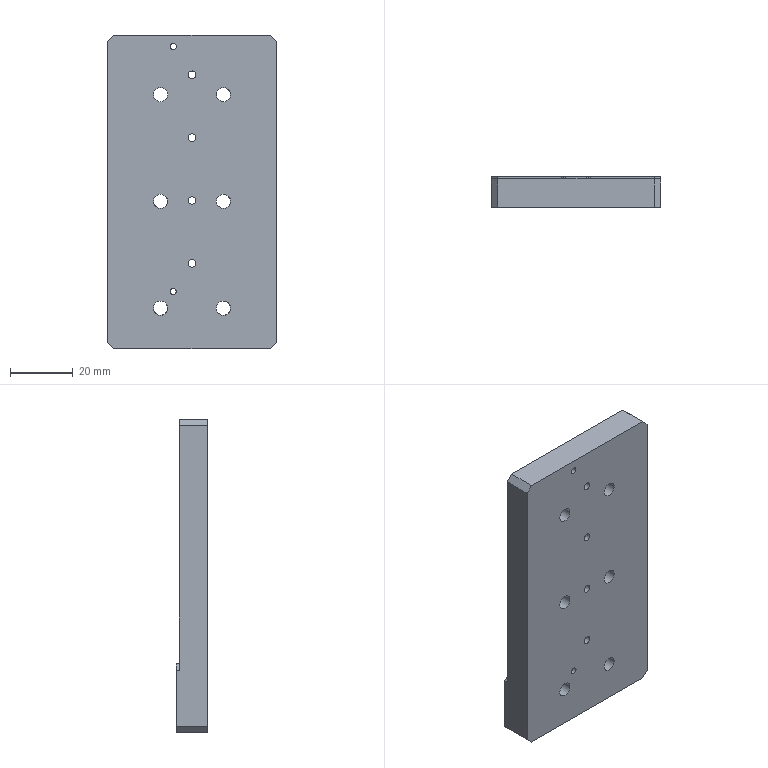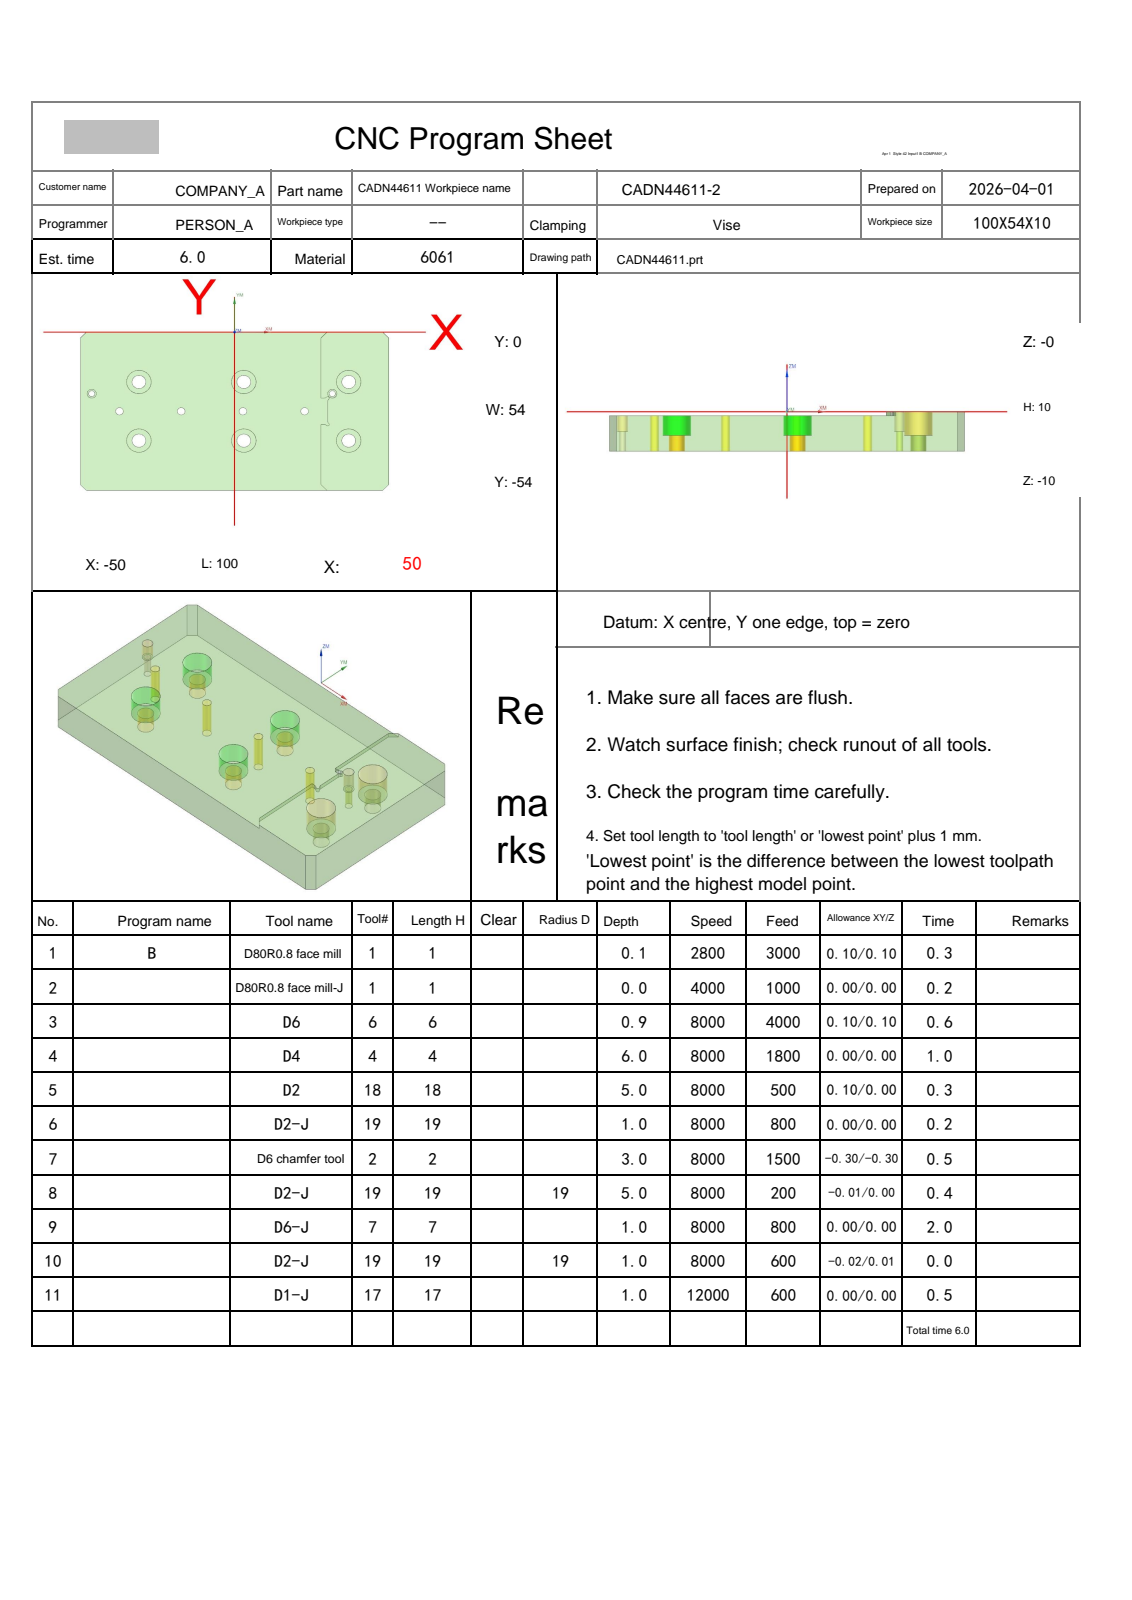NC program | NX | posted by the shop | part box 54 x 10 x 100 mm
Lines 1 to 1970 of 3760, first 1655 of 1968 lines:
%
O0001
(Machine time: 8.37 MIN)
(===Total Tool:8===)
(T1=D80R0.8 face mill D=80.  R=0.8  D-  H01 Z=-0.   )
(T6=D6      D=6.   R=0.   D-  H06 Z=-0.9  )
(T4=D4      D=4.   R=0.   D-  H04 Z=-6.   )
(T18=D2     D=2.   R=0.   D-  H18 Z=-5.   )
(T19=D2-J   D=2.   R=0.   D-  H19 Z=-5.   )
(T2=D6 chamfer tool   D=6.   R=0.   D-  H02 Z=-3.   )
(T7=D6-J    D=6.   R=0.   D7  H07 Z=-1.   )
(T17=D1-J   D=0.96 R=0.   D-  H17 Z=-1.   )
G80 G90 G17 G49 G40
G91 G28 Z0
M01
N1 T01 M06
(D80R0.8 face mill  D=80. R=0.8 H=01 ce=0.10 di=0.10)
G00 G90 G54 X-102.097 Y-27. M03 S2800
G43 H01 Z20.
M08
Z3.525
G01 Z1.525 F3000.
X-90.097
X90.097
X102.097
Z3.525
G00 X-102.097
Z3.05
G01 Z1.05
X-90.097
X90.097
X102.097
Z3.05
G00 X-102.097
Z2.575
G01 Z.575
X-90.097
X90.097
X102.097
Z2.575
G00 X-102.097
Z2.1
G01 Z.1
X-90.097
X90.097
X102.097
Z2.1
G00 Z20.
G91 G28 Z0.0
M05
M09
G91 G28 Z0.0
M01
N2 T01 M06
(D80R0.8 face mill-J  D=80. R=0.8 H=01 ce=0.00 di=0.00)
G00 G90 G54 X-101.999 Y-27. M03 S4000
G43 H01 Z20.
M08
Z2.
G01 Z0.0 F1000.
X-89.999
X89.999
X101.999
Z2.
G00 Z20.
G91 G28 Z0.0
M05
M09
G91 G28 Z0.0
M01
N3 T06 M06
(D6  D=6. R=0. H=06 ce=0.10 di=0.10)
G00 G90 G54 X-51.515 Y4.97 M03 S8000
G43 H06 Z11.801
M08
Z1.05
G01 Z-.45 F4000.
X-51.589 Y.569
G03 X-51.6 Y-.716 I76.489 J-1.285
G01 Y-25.601
G03 X-51.587 Y-27.001 I76.5 J0.0
X-51.6 Y-28.401 I76.487 J-1.4
G01 Y-53.291
G03 X-51.593 Y-54.325 I76.5 J.007
X-51.417 Y-54.74 I.6 J.008
G01 X-49.393 Y-56.764
G03 X-48.969 Y-56.94 I.424 J.424
G01 X-47.573
G03 X-47.033 Y-56.4 I0.0 J.54
G01 X-47.034 Y-56.377
G02 X-47.1 Y-53.291 I71.934 J3.093
G01 Y-28.401
G02 X-47.086 Y-27.001 I72. J0.0
X-47.1 Y-25.601 I71.986 J1.4
G01 Y-.716
G02 X-47.034 Y2.366 I72. J0.0
X-46.435 Y2.94 I.599 J-.026
G01 X-43.068
G02 X-42.529 Y2.4 I0.0 J-.54
G01 Y2.376
G03 X-42.6 Y-.716 I67.429 J-3.092
G01 Y-25.601
G03 X-42.585 Y-27.001 I67.5 J0.0
X-42.6 Y-28.401 I67.485 J-1.4
G01 Y-53.29
G03 X-42.53 Y-56.368 I67.5 J.006
X-41.93 Y-56.94 I.599 J.028
G01 X-38.563
G03 X-38.024 Y-56.4 I0.0 J.54
G01 Y-56.374
G02 X-38.1 Y-53.29 I62.924 J3.09
G01 Y-28.401
G02 X-38.084 Y-27.001 I63. J0.0
X-38.1 Y-25.601 I62.984 J1.4
G01 Y-.716
G02 X-38.024 Y2.37 I63. J0.0
X-37.425 Y2.94 I.599 J-.03
G01 X-34.057
G02 X-33.518 Y2.4 I0.0 J-.54
G01 Y2.372
G03 X-33.6 Y-.716 I58.418 J-3.088
G01 Y-25.601
G03 X-33.583 Y-27.001 I58.5 J0.0
X-33.6 Y-28.401 I58.483 J-1.4
G01 Y-53.29
G03 X-33.518 Y-56.372 I58.5 J.005
X-32.92 Y-56.94 I.599 J.032
G01 X-29.551
G03 X-29.011 Y-56.4 I0.0 J.54
G01 X-29.012 Y-56.369
G02 X-29.1 Y-53.289 I53.912 J3.085
G01 Y-28.401
G02 X-29.082 Y-27.001 I54. J0.0
X-29.1 Y-25.601 I53.982 J1.4
G01 Y-.716
G02 X-29.011 Y2.375 I54. J0.0
X-28.413 Y2.94 I.599 J-.035
G01 X-25.043
G02 X-24.503 Y2.4 I0.0 J-.54
G01 X-24.504 Y2.367
G03 X-24.6 Y-.716 I49.404 J-3.083
G01 Y-25.601
G03 X-24.58 Y-27.001 I49.5 J0.0
X-24.6 Y-28.401 I49.48 J-1.4
G01 Y-53.289
G03 X-24.503 Y-56.378 I49.5 J.005
X-23.905 Y-56.94 I.599 J.038
G01 X-20.533
G03 X-19.993 Y-56.4 I0.0 J.54
G01 X-19.995 Y-56.363
G02 X-20.1 Y-53.288 I44.895 J3.079
G01 Y-28.401
G02 X-20.078 Y-27.001 I45. J0.0
X-20.1 Y-25.601 I44.978 J1.4
G01 Y-.716
G02 X-19.993 Y2.382 I45. J0.0
X-19.395 Y2.94 I.599 J-.042
G01 X-16.021
G02 X-15.482 Y2.4 I0.0 J-.54
G01 X-15.483 Y2.359
G03 X-15.6 Y-.716 I40.383 J-3.075
G01 Y-25.601
G03 X-15.576 Y-27.001 I40.5 J0.0
X-15.6 Y-28.401 I40.476 J-1.4
G01 Y-53.288
G03 X-15.481 Y-56.386 I40.5 J.004
X-14.883 Y-56.94 I.598 J.046
G01 X-11.507
G03 X-10.967 Y-56.4 I0.0 J.54
G01 X-10.969 Y-56.354
G02 X-11.1 Y-53.287 I35.869 J3.07
G01 Y-28.401
G02 X-11.073 Y-27.001 I36. J0.0
X-11.1 Y-25.601 I35.973 J1.4
G01 Y-.716
G02 X-10.966 Y2.392 I36. J0.0
X-10.368 Y2.94 I.598 J-.052
G01 X-6.922
G02 X-6.442 Y2.46 I0.0 J-.48
G01 X-6.444 Y2.413
G03 X-6.6 Y-.716 I31.344 J-3.129
G01 Y-25.601
G03 X-6.569 Y-27.001 I31.5 J0.0
X-6.6 Y-28.401 I31.469 J-1.4
G01 Y-53.287
G03 X-6.446 Y-56.4 I31.5 J.003
X-5.849 Y-56.94 I.597 J.06
G01 X-2.396
G03 X-1.916 Y-56.46 I0.0 J.48
G01 X-1.919 Y-56.405
G02 X-2.1 Y-53.287 I26.819 J3.121
G01 Y-28.401
G02 X-2.065 Y-27.029 I27. J0.0
G01 Y-26.974
G02 X-2.1 Y-25.601 I26.965 J1.372
G01 Y-.716
G02 X-1.918 Y2.41 I27. J0.0
X-1.323 Y2.94 I.596 J-.07
G01 X2.141
G02 X2.621 Y2.46 I0.0 J-.48
G01 X2.616 Y2.394
G03 X2.4 Y-.716 I22.284 J-3.11
G01 Y-25.601
G03 X2.442 Y-26.967 I22.5 J0.0
G01 Y-27.035
G03 X2.4 Y-28.401 I22.458 J-1.366
G01 Y-53.286
G03 X2.62 Y-56.424 I22.5 J.002
X3.214 Y-56.94 I.594 J.084
G01 X6.695
G03 X7.175 Y-56.46 I0.0 J.48
G01 X7.168 Y-56.378
G02 X6.9 Y-53.286 I17.732 J3.094
G01 Y-28.401
G02 X6.951 Y-27.044 I18. J0.0
G01 Y-26.958
G02 X6.9 Y-25.601 I17.949 J1.357
G01 Y-.716
G02 X7.18 Y2.446 I18. J0.0
X7.77 Y2.94 I.591 J-.106
G01 X11.362
G02 X11.781 Y2.52 I0.0 J-.42
G01 X11.77 Y2.423
G03 X11.4 Y-.716 I13.13 J-3.139
G01 Y-25.601
G03 X11.467 Y-26.944 I13.5 J0.0
G01 Y-27.059
G03 X11.4 Y-28.401 I13.433 J-1.343
G01 Y-53.285
G03 X11.784 Y-56.482 I13.5 J.001
X12.367 Y-56.94 I.583 J.142
G01 X16.14
G03 X16.499 Y-56.58 I0.0 J.36
G01 X16.477 Y-56.453
G02 X15.9 Y-53.285 I8.423 J3.169
G01 Y-28.401
G02 X15.996 Y-27.087 I9. J0.0
G01 X16.023 Y-27.001
X15.996 Y-26.916
G02 X15.9 Y-25.601 I8.904 J1.314
G01 Y-.716
G02 X16.517 Y2.558 I9. J0.0
X17.075 Y2.94 I.559 J-.218
G01 X21.613
G02 X21.853 Y2.7 I0.0 J-.24
G01 X21.782 Y2.53
X21.718 Y2.466
G03 X20.4 Y-.716 I3.182 J-3.182
G01 Y-25.601
G03 X20.573 Y-26.838 I4.5 J0.0
G01 X20.596 Y-27.001
X20.573 Y-27.164
G03 X20.4 Y-28.401 I4.327 J-1.237
G01 Y-53.284
G03 X21.718 Y-56.466 I4.5 J0.0
G01 X22.058 Y-56.806
G03 X22.379 Y-56.973 I.424 J.424
G01 X28.029 Y-57.955
X28.132 Y-57.964
G03 X28.732 Y-57.364 I0.0 J.6
X28.556 Y-56.94 I-.6 J0.0
G01 X24.9 Y-53.284
Y-28.401
X27.101
Y-25.601
X24.9
Y-.716
X28.556 Y2.94
X31.716 Y6.1
Z1.05
G00 X-51.515 Y4.97
Z.6
G01 Z-.9
X-51.589 Y.569
G03 X-51.6 Y-.716 I76.489 J-1.285
G01 Y-25.601
G03 X-51.587 Y-27.001 I76.5 J0.0
X-51.6 Y-28.401 I76.487 J-1.4
G01 Y-53.291
G03 X-51.593 Y-54.325 I76.5 J.007
X-51.417 Y-54.74 I.6 J.008
G01 X-49.393 Y-56.764
G03 X-48.969 Y-56.94 I.424 J.424
G01 X-47.573
G03 X-47.033 Y-56.4 I0.0 J.54
G01 X-47.034 Y-56.377
G02 X-47.1 Y-53.291 I71.934 J3.093
G01 Y-28.401
G02 X-47.086 Y-27.001 I72. J0.0
X-47.1 Y-25.601 I71.986 J1.4
G01 Y-.716
G02 X-47.034 Y2.366 I72. J0.0
X-46.435 Y2.94 I.599 J-.026
G01 X-43.068
G02 X-42.529 Y2.4 I0.0 J-.54
G01 Y2.376
G03 X-42.6 Y-.716 I67.429 J-3.092
G01 Y-25.601
G03 X-42.585 Y-27.001 I67.5 J0.0
X-42.6 Y-28.401 I67.485 J-1.4
G01 Y-53.29
G03 X-42.53 Y-56.368 I67.5 J.006
X-41.93 Y-56.94 I.599 J.028
G01 X-38.563
G03 X-38.024 Y-56.4 I0.0 J.54
G01 Y-56.374
G02 X-38.1 Y-53.29 I62.924 J3.09
G01 Y-28.401
G02 X-38.084 Y-27.001 I63. J0.0
X-38.1 Y-25.601 I62.984 J1.4
G01 Y-.716
G02 X-38.024 Y2.37 I63. J0.0
X-37.425 Y2.94 I.599 J-.03
G01 X-34.057
G02 X-33.518 Y2.4 I0.0 J-.54
G01 Y2.372
G03 X-33.6 Y-.716 I58.418 J-3.088
G01 Y-25.601
G03 X-33.583 Y-27.001 I58.5 J0.0
X-33.6 Y-28.401 I58.483 J-1.4
G01 Y-53.29
G03 X-33.518 Y-56.372 I58.5 J.005
X-32.92 Y-56.94 I.599 J.032
G01 X-29.551
G03 X-29.011 Y-56.4 I0.0 J.54
G01 X-29.012 Y-56.369
G02 X-29.1 Y-53.289 I53.912 J3.085
G01 Y-28.401
G02 X-29.082 Y-27.001 I54. J0.0
X-29.1 Y-25.601 I53.982 J1.4
G01 Y-.716
G02 X-29.011 Y2.375 I54. J0.0
X-28.413 Y2.94 I.599 J-.035
G01 X-25.043
G02 X-24.503 Y2.4 I0.0 J-.54
G01 X-24.504 Y2.367
G03 X-24.6 Y-.716 I49.404 J-3.083
G01 Y-25.601
G03 X-24.58 Y-27.001 I49.5 J0.0
X-24.6 Y-28.401 I49.48 J-1.4
G01 Y-53.289
G03 X-24.503 Y-56.378 I49.5 J.005
X-23.905 Y-56.94 I.599 J.038
G01 X-20.533
G03 X-19.993 Y-56.4 I0.0 J.54
G01 X-19.995 Y-56.363
G02 X-20.1 Y-53.288 I44.895 J3.079
G01 Y-28.401
G02 X-20.078 Y-27.001 I45. J0.0
X-20.1 Y-25.601 I44.978 J1.4
G01 Y-.716
G02 X-19.993 Y2.382 I45. J0.0
X-19.395 Y2.94 I.599 J-.042
G01 X-16.021
G02 X-15.482 Y2.4 I0.0 J-.54
G01 X-15.483 Y2.359
G03 X-15.6 Y-.716 I40.383 J-3.075
G01 Y-25.601
G03 X-15.576 Y-27.001 I40.5 J0.0
X-15.6 Y-28.401 I40.476 J-1.4
G01 Y-53.288
G03 X-15.481 Y-56.386 I40.5 J.004
X-14.883 Y-56.94 I.598 J.046
G01 X-11.507
G03 X-10.967 Y-56.4 I0.0 J.54
G01 X-10.969 Y-56.354
G02 X-11.1 Y-53.287 I35.869 J3.07
G01 Y-28.401
G02 X-11.073 Y-27.001 I36. J0.0
X-11.1 Y-25.601 I35.973 J1.4
G01 Y-.716
G02 X-10.966 Y2.392 I36. J0.0
X-10.368 Y2.94 I.598 J-.052
G01 X-6.922
G02 X-6.442 Y2.46 I0.0 J-.48
G01 X-6.444 Y2.413
G03 X-6.6 Y-.716 I31.344 J-3.129
G01 Y-25.601
G03 X-6.569 Y-27.001 I31.5 J0.0
X-6.6 Y-28.401 I31.469 J-1.4
G01 Y-53.287
G03 X-6.446 Y-56.4 I31.5 J.003
X-5.849 Y-56.94 I.597 J.06
G01 X-2.396
G03 X-1.916 Y-56.46 I0.0 J.48
G01 X-1.919 Y-56.405
G02 X-2.1 Y-53.287 I26.819 J3.121
G01 Y-28.401
G02 X-2.065 Y-27.029 I27. J0.0
G01 Y-26.974
G02 X-2.1 Y-25.601 I26.965 J1.372
G01 Y-.716
G02 X-1.918 Y2.41 I27. J0.0
X-1.323 Y2.94 I.596 J-.07
G01 X2.141
G02 X2.621 Y2.46 I0.0 J-.48
G01 X2.616 Y2.394
G03 X2.4 Y-.716 I22.284 J-3.11
G01 Y-25.601
G03 X2.442 Y-26.967 I22.5 J0.0
G01 Y-27.035
G03 X2.4 Y-28.401 I22.458 J-1.366
G01 Y-53.286
G03 X2.62 Y-56.424 I22.5 J.002
X3.214 Y-56.94 I.594 J.084
G01 X6.695
G03 X7.175 Y-56.46 I0.0 J.48
G01 X7.168 Y-56.378
G02 X6.9 Y-53.286 I17.732 J3.094
G01 Y-28.401
G02 X6.951 Y-27.044 I18. J0.0
G01 Y-26.958
G02 X6.9 Y-25.601 I17.949 J1.357
G01 Y-.716
G02 X7.18 Y2.446 I18. J0.0
X7.77 Y2.94 I.591 J-.106
G01 X11.362
G02 X11.781 Y2.52 I0.0 J-.42
G01 X11.77 Y2.423
G03 X11.4 Y-.716 I13.13 J-3.139
G01 Y-25.601
G03 X11.467 Y-26.944 I13.5 J0.0
G01 Y-27.059
G03 X11.4 Y-28.401 I13.433 J-1.343
G01 Y-53.285
G03 X11.784 Y-56.482 I13.5 J.001
X12.367 Y-56.94 I.583 J.142
G01 X16.14
G03 X16.499 Y-56.58 I0.0 J.36
G01 X16.477 Y-56.453
G02 X15.9 Y-53.285 I8.423 J3.169
G01 Y-28.401
G02 X15.996 Y-27.087 I9. J0.0
G01 X16.023 Y-27.001
X15.996 Y-26.916
G02 X15.9 Y-25.601 I8.904 J1.314
G01 Y-.716
G02 X16.517 Y2.558 I9. J0.0
X17.075 Y2.94 I.559 J-.218
G01 X21.613
G02 X21.853 Y2.7 I0.0 J-.24
G01 X21.782 Y2.53
X21.718 Y2.466
G03 X20.4 Y-.716 I3.182 J-3.182
G01 Y-25.601
G03 X20.573 Y-26.838 I4.5 J0.0
G01 X20.596 Y-27.001
X20.573 Y-27.164
G03 X20.4 Y-28.401 I4.327 J-1.237
G01 Y-53.284
G03 X21.718 Y-56.466 I4.5 J0.0
G01 X22.058 Y-56.806
G03 X22.379 Y-56.973 I.424 J.424
G01 X28.029 Y-57.955
X28.132 Y-57.964
G03 X28.732 Y-57.364 I0.0 J.6
X28.556 Y-56.94 I-.6 J0.0
G01 X24.9 Y-53.284
Y-28.401
X27.101
Y-25.601
X24.9
Y-.716
X28.556 Y2.94
X31.716 Y6.1
Z.6
G00 Z11.801
G91 G28 Z0.0
M05
M09
G91 G28 Z0.0
M01
N4 T04 M06
(D4  D=4. R=0. H=04 ce=0.07 di=0.00)
G00 G90 G54 X3. Y-37. M03 S8000
G43 H04 Z20.
M08
Z-.7
G03 X2.035 Y-36.035 I-.965 J0.0 F1800.
X1.07 Y-37. I0.0 J-.965
X1.07 Y-37. Z-1.05 I1.93 J0.0
X1.07 Y-37. Z-1.4 I1.93 J0.0
X1.07 Y-37. Z-1.75 I1.93 J0.0
X1.07 Y-37. Z-2.1 I1.93 J0.0
X1.07 Y-37. Z-2.45 I1.93 J0.0
X1.07 Y-37. Z-2.8 I1.93 J0.0
X1.07 Y-37. Z-3.15 I1.93 J0.0
X1.07 Y-37. Z-3.5 I1.93 J0.0
X1.07 Y-37. Z-3.85 I1.93 J0.0
X1.07 Y-37. Z-4.2 I1.93 J0.0
X1.07 Y-37. Z-4.55 I1.93 J0.0
X1.07 Y-37. Z-4.9 I1.93 J0.0
X1.07 Y-37. Z-5.25 I1.93 J0.0
X1.07 Y-37. Z-5.6 I1.93 J0.0
X1.07 Y-37. Z-5.95 I1.93 J0.0
X1.797 Y-38.509 Z-6. I1.93 J0.0
X3. Y-38.93 I1.203 J1.509
X4.93 Y-37. I0.0 J1.93
X3. Y-35.07 I-1.93 J0.0
X1.07 Y-37. I0.0 J-1.93
X1.797 Y-38.509 I1.93 J0.0
X2.398 Y-38.719 I.602 J.754
X3.363 Y-37.754 I0.0 J.965
X3. Y-37. I-.965 J0.0
G00 Z20.
Y-17.
Z-.7
G03 X2.035 Y-16.035 I-.965 J0.0
X1.07 Y-17. I0.0 J-.965
X1.07 Y-17. Z-1.05 I1.93 J0.0
X1.07 Y-17. Z-1.4 I1.93 J0.0
X1.07 Y-17. Z-1.75 I1.93 J0.0
X1.07 Y-17. Z-2.1 I1.93 J0.0
X1.07 Y-17. Z-2.45 I1.93 J0.0
X1.07 Y-17. Z-2.8 I1.93 J0.0
X1.07 Y-17. Z-3.15 I1.93 J0.0
X1.07 Y-17. Z-3.5 I1.93 J0.0
X1.07 Y-17. Z-3.85 I1.93 J0.0
X1.07 Y-17. Z-4.2 I1.93 J0.0
X1.07 Y-17. Z-4.55 I1.93 J0.0
X1.07 Y-17. Z-4.9 I1.93 J0.0
X1.07 Y-17. Z-5.25 I1.93 J0.0
X1.07 Y-17. Z-5.6 I1.93 J0.0
X1.07 Y-17. Z-5.95 I1.93 J0.0
X1.797 Y-18.509 Z-6. I1.93 J0.0
X3. Y-18.93 I1.203 J1.509
X4.93 Y-17. I0.0 J1.93
X3. Y-15.07 I-1.93 J0.0
X1.07 Y-17. I0.0 J-1.93
X1.797 Y-18.509 I1.93 J0.0
X2.398 Y-18.719 I.602 J.754
X3.363 Y-17.754 I0.0 J.965
X3. Y-17. I-.965 J0.0
G00 Z20.
X-31.
Z-.7
G03 X-31.965 Y-16.035 I-.965 J0.0
X-32.93 Y-17. I0.0 J-.965
X-32.93 Y-17. Z-1.05 I1.93 J0.0
X-32.93 Y-17. Z-1.4 I1.93 J0.0
X-32.93 Y-17. Z-1.75 I1.93 J0.0
X-32.93 Y-17. Z-2.1 I1.93 J0.0
X-32.93 Y-17. Z-2.45 I1.93 J0.0
X-32.93 Y-17. Z-2.8 I1.93 J0.0
X-32.93 Y-17. Z-3.15 I1.93 J0.0
X-32.93 Y-17. Z-3.5 I1.93 J0.0
X-32.93 Y-17. Z-3.85 I1.93 J0.0
X-32.93 Y-17. Z-4.2 I1.93 J0.0
X-32.93 Y-17. Z-4.55 I1.93 J0.0
X-32.93 Y-17. Z-4.9 I1.93 J0.0
X-32.93 Y-17. Z-5.25 I1.93 J0.0
X-32.93 Y-17. Z-5.6 I1.93 J0.0
X-32.93 Y-17. Z-5.95 I1.93 J0.0
X-32.203 Y-18.509 Z-6. I1.93 J0.0
X-31. Y-18.93 I1.203 J1.509
X-29.07 Y-17. I0.0 J1.93
X-31. Y-15.07 I-1.93 J0.0
X-32.93 Y-17. I0.0 J-1.93
X-32.203 Y-18.509 I1.93 J0.0
X-31.602 Y-18.719 I.602 J.754
X-30.637 Y-17.754 I0.0 J.965
X-31. Y-17. I-.965 J0.0
G00 Z20.
Y-37.
Z-.7
G03 X-31.965 Y-36.035 I-.965 J0.0
X-32.93 Y-37. I0.0 J-.965
X-32.93 Y-37. Z-1.05 I1.93 J0.0
X-32.93 Y-37. Z-1.4 I1.93 J0.0
X-32.93 Y-37. Z-1.75 I1.93 J0.0
X-32.93 Y-37. Z-2.1 I1.93 J0.0
X-32.93 Y-37. Z-2.45 I1.93 J0.0
X-32.93 Y-37. Z-2.8 I1.93 J0.0
X-32.93 Y-37. Z-3.15 I1.93 J0.0
X-32.93 Y-37. Z-3.5 I1.93 J0.0
X-32.93 Y-37. Z-3.85 I1.93 J0.0
X-32.93 Y-37. Z-4.2 I1.93 J0.0
X-32.93 Y-37. Z-4.55 I1.93 J0.0
X-32.93 Y-37. Z-4.9 I1.93 J0.0
X-32.93 Y-37. Z-5.25 I1.93 J0.0
X-32.93 Y-37. Z-5.6 I1.93 J0.0
X-32.93 Y-37. Z-5.95 I1.93 J0.0
X-32.203 Y-38.509 Z-6. I1.93 J0.0
X-31. Y-38.93 I1.203 J1.509
X-29.07 Y-37. I0.0 J1.93
X-31. Y-35.07 I-1.93 J0.0
X-32.93 Y-37. I0.0 J-1.93
X-32.203 Y-38.509 I1.93 J0.0
X-31.602 Y-38.719 I.602 J.754
X-30.637 Y-37.754 I0.0 J.965
X-31. Y-37. I-.965 J0.0
G00 Z20.
G00 G90 X37. Y-17. M03 S8000
Z20.
Z.3
G03 X36.035 Y-16.035 I-.965 J0.0 F1800.
X35.07 Y-17. I0.0 J-.965
X35.07 Y-17. Z-.05 I1.93 J0.0
X35.07 Y-17. Z-.4 I1.93 J0.0
X35.07 Y-17. Z-.75 I1.93 J0.0
X35.07 Y-17. Z-1.1 I1.93 J0.0
X35.07 Y-17. Z-1.45 I1.93 J0.0
X35.07 Y-17. Z-1.8 I1.93 J0.0
X35.07 Y-17. Z-2.15 I1.93 J0.0
X35.07 Y-17. Z-2.5 I1.93 J0.0
X35.07 Y-17. Z-2.85 I1.93 J0.0
X35.07 Y-17. Z-3.2 I1.93 J0.0
X35.07 Y-17. Z-3.55 I1.93 J0.0
X35.07 Y-17. Z-3.9 I1.93 J0.0
X35.07 Y-17. Z-4.25 I1.93 J0.0
X35.07 Y-17. Z-4.6 I1.93 J0.0
X35.07 Y-17. Z-4.95 I1.93 J0.0
X35.07 Y-17. Z-5.3 I1.93 J0.0
X35.07 Y-17. Z-5.65 I1.93 J0.0
X35.07 Y-17. Z-6. I1.93 J0.0
X37. Y-18.93 I1.93 J0.0
X38.93 Y-17. I0.0 J1.93
X37. Y-15.07 I-1.93 J0.0
X35.07 Y-17. I0.0 J-1.93
X36.035 Y-17.965 I.965 J0.0
X37. Y-17. I0.0 J.965
G00 Z20.
Y-37.
Z.3
G03 X36.035 Y-36.035 I-.965 J0.0
X35.07 Y-37. I0.0 J-.965
X35.07 Y-37. Z-.05 I1.93 J0.0
X35.07 Y-37. Z-.4 I1.93 J0.0
X35.07 Y-37. Z-.75 I1.93 J0.0
X35.07 Y-37. Z-1.1 I1.93 J0.0
X35.07 Y-37. Z-1.45 I1.93 J0.0
X35.07 Y-37. Z-1.8 I1.93 J0.0
X35.07 Y-37. Z-2.15 I1.93 J0.0
X35.07 Y-37. Z-2.5 I1.93 J0.0
X35.07 Y-37. Z-2.85 I1.93 J0.0
X35.07 Y-37. Z-3.2 I1.93 J0.0
X35.07 Y-37. Z-3.55 I1.93 J0.0
X35.07 Y-37. Z-3.9 I1.93 J0.0
X35.07 Y-37. Z-4.25 I1.93 J0.0
X35.07 Y-37. Z-4.6 I1.93 J0.0
X35.07 Y-37. Z-4.95 I1.93 J0.0
X35.07 Y-37. Z-5.3 I1.93 J0.0
X35.07 Y-37. Z-5.65 I1.93 J0.0
X35.07 Y-37. Z-6. I1.93 J0.0
X37. Y-38.93 I1.93 J0.0
X38.93 Y-37. I0.0 J1.93
X37. Y-35.07 I-1.93 J0.0
X35.07 Y-37. I0.0 J-1.93
X36.035 Y-37.965 I.965 J0.0
X37. Y-37. I0.0 J.965
G00 Z20.
G00 G90 X3. Y-37. M03 S8000
Z20.
Z-6.
G01 X1.404 Y-36.671 F600.
X1.336 Y-36.664
G03 X1. Y-37. I0.0 J-.336
X3. Y-39. I2. J0.0
X5. Y-37. I0.0 J2.
X3. Y-35. I-2. J0.0
X1. Y-37. I0.0 J-2.
X1.062 Y-37.495 I2. J0.0
X1.388 Y-37.748 I.325 J.083
G01 X1.535 Y-37.714
X3. Y-37.
G00 Z20.
Y-17.
Z-6.
G01 X1.404 Y-16.671
X1.336 Y-16.664
G03 X1. Y-17. I0.0 J-.336
X3. Y-19. I2. J0.0
X5. Y-17. I0.0 J2.
X3. Y-15. I-2. J0.0
X1. Y-17. I0.0 J-2.
X1.062 Y-17.495 I2. J0.0
X1.388 Y-17.748 I.325 J.083
G01 X1.535 Y-17.714
X3. Y-17.
G00 Z20.
X-31.
Z-6.
G01 X-32.596 Y-16.671
X-32.664 Y-16.664
G03 X-33. Y-17. I0.0 J-.336
X-31. Y-19. I2. J0.0
X-29. Y-17. I0.0 J2.
X-31. Y-15. I-2. J0.0
X-33. Y-17. I0.0 J-2.
X-32.938 Y-17.495 I2. J0.0
X-32.612 Y-17.748 I.325 J.083
G01 X-32.465 Y-17.714
X-31. Y-17.
G00 Z20.
Y-37.
Z-6.
G01 X-32.596 Y-36.671
X-32.664 Y-36.664
G03 X-33. Y-37. I0.0 J-.336
X-31. Y-39. I2. J0.0
X-29. Y-37. I0.0 J2.
X-31. Y-35. I-2. J0.0
X-33. Y-37. I0.0 J-2.
X-32.938 Y-37.495 I2. J0.0
X-32.612 Y-37.748 I.325 J.083
G01 X-32.465 Y-37.714
X-31. Y-37.
G00 Z20.
G00 G90 X37. Y-17. M03 S8000
Z20.
Z-3.
G01 X35.404 Y-16.671 F600.
X35.336 Y-16.664
G03 X35. Y-17. I0.0 J-.336
X37. Y-19. I2. J0.0
X39. Y-17. I0.0 J2.
X37. Y-15. I-2. J0.0
X35. Y-17. I0.0 J-2.
X35.062 Y-17.495 I2. J0.0
X35.388 Y-17.748 I.325 J.083
G01 X35.535 Y-17.714
X37. Y-17.
Z-6. F10000.
X35.404 Y-16.671 F600.
X35.336 Y-16.664
G03 X35. Y-17. I0.0 J-.336
X37. Y-19. I2. J0.0
X39. Y-17. I0.0 J2.
X37. Y-15. I-2. J0.0
X35. Y-17. I0.0 J-2.
X35.062 Y-17.495 I2. J0.0
X35.388 Y-17.748 I.325 J.083
G01 X35.535 Y-17.714
X37. Y-17.
G00 Z20.
Y-37.
Z-3.
G01 X35.404 Y-36.671
X35.336 Y-36.664
G03 X35. Y-37. I0.0 J-.336
X37. Y-39. I2. J0.0
X39. Y-37. I0.0 J2.
X37. Y-35. I-2. J0.0
X35. Y-37. I0.0 J-2.
X35.062 Y-37.495 I2. J0.0
X35.388 Y-37.748 I.325 J.083
G01 X35.535 Y-37.714
X37. Y-37.
Z-6. F10000.
X35.404 Y-36.671 F600.
X35.336 Y-36.664
G03 X35. Y-37. I0.0 J-.336
X37. Y-39. I2. J0.0
X39. Y-37. I0.0 J2.
X37. Y-35. I-2. J0.0
X35. Y-37. I0.0 J-2.
X35.062 Y-37.495 I2. J0.0
X35.388 Y-37.748 I.325 J.083
G01 X35.535 Y-37.714
X37. Y-37.
G00 Z20.
G91 G28 Z0.0
M05
M09
G91 G28 Z0.0
M01
N5 T18 M06
(D2  D=2. R=0. H=18 ce=0.10 di=0.00)
G00 G90 G54 X-46.299 Y-21. M03 S8000
G43 H18 Z20.
M08
Z-.7
G03 X-46.499 Y-20.8 I-.2 J0.0 F500.
X-46.699 Y-21. I0.0 J-.2
X-46.699 Y-21. Z-.85 I.4 J0.0
X-46.699 Y-21. Z-1. I.4 J0.0
X-46.699 Y-21. Z-1.15 I.4 J0.0
X-46.699 Y-21. Z-1.3 I.4 J0.0
X-46.699 Y-21. Z-1.45 I.4 J0.0
X-46.699 Y-21. Z-1.6 I.4 J0.0
X-46.699 Y-21. Z-1.75 I.4 J0.0
X-46.699 Y-21. Z-1.9 I.4 J0.0
X-46.699 Y-21. Z-2.05 I.4 J0.0
X-46.699 Y-21. Z-2.2 I.4 J0.0
X-46.699 Y-21. Z-2.35 I.4 J0.0
X-46.699 Y-21. Z-2.5 I.4 J0.0
X-46.699 Y-21. Z-2.65 I.4 J0.0
X-46.699 Y-21. Z-2.8 I.4 J0.0
X-46.699 Y-21. Z-2.95 I.4 J0.0
X-46.699 Y-21. Z-3.1 I.4 J0.0
X-46.699 Y-21. Z-3.25 I.4 J0.0
X-46.699 Y-21. Z-3.4 I.4 J0.0
X-46.699 Y-21. Z-3.55 I.4 J0.0
X-46.699 Y-21. Z-3.7 I.4 J0.0
X-46.699 Y-21. Z-3.85 I.4 J0.0
X-46.699 Y-21. Z-4. I.4 J0.0
X-46.699 Y-21. Z-4.15 I.4 J0.0
X-46.699 Y-21. Z-4.3 I.4 J0.0
X-46.699 Y-21. Z-4.45 I.4 J0.0
X-46.699 Y-21. Z-4.6 I.4 J0.0
X-46.699 Y-21. Z-4.75 I.4 J0.0
X-46.699 Y-21. Z-4.9 I.4 J0.0
X-46.097 Y-20.655 Z-5. I.4 J0.0
X-46.299 Y-20.6 I-.202 J-.345
X-46.699 Y-21. I0.0 J-.4
X-46.299 Y-21.4 I.4 J0.0
X-45.899 Y-21. I0.0 J.4
X-46.097 Y-20.655 I-.4 J0.0
G01 X-46.198 Y-20.627
G03 X-46.398 Y-20.827 I0.0 J-.2
X-46.299 Y-21. I.2 J0.0
G00 Z20.
G00 G90 X31.701 Y-21. M03 S8000
Z20.
Z.3
G03 X31.501 Y-20.8 I-.2 J0.0 F500.
X31.301 Y-21. I0.0 J-.2
X31.301 Y-21. Z.15 I.4 J0.0
X31.301 Y-21. Z0.0 I.4 J0.0
X31.301 Y-21. Z-.15 I.4 J0.0
X31.301 Y-21. Z-.3 I.4 J0.0
X31.301 Y-21. Z-.45 I.4 J0.0
X31.301 Y-21. Z-.6 I.4 J0.0
X31.301 Y-21. Z-.75 I.4 J0.0
X31.301 Y-21. Z-.9 I.4 J0.0
X31.301 Y-21. Z-1.05 I.4 J0.0
X31.301 Y-21. Z-1.2 I.4 J0.0
X31.301 Y-21. Z-1.35 I.4 J0.0
X31.301 Y-21. Z-1.5 I.4 J0.0
X31.301 Y-21. Z-1.65 I.4 J0.0
X31.301 Y-21. Z-1.8 I.4 J0.0
X31.301 Y-21. Z-1.95 I.4 J0.0
X31.301 Y-21. Z-2.1 I.4 J0.0
X31.301 Y-21. Z-2.25 I.4 J0.0
X31.301 Y-21. Z-2.4 I.4 J0.0
X31.301 Y-21. Z-2.55 I.4 J0.0
X31.301 Y-21. Z-2.7 I.4 J0.0
X31.301 Y-21. Z-2.85 I.4 J0.0
X31.301 Y-21. Z-3. I.4 J0.0
X31.301 Y-21. Z-3.15 I.4 J0.0
X31.301 Y-21. Z-3.3 I.4 J0.0
X31.301 Y-21. Z-3.45 I.4 J0.0
X31.301 Y-21. Z-3.6 I.4 J0.0
X31.301 Y-21. Z-3.75 I.4 J0.0
X31.301 Y-21. Z-3.9 I.4 J0.0
X31.301 Y-21. Z-4.05 I.4 J0.0
X31.301 Y-21. Z-4.2 I.4 J0.0
X31.301 Y-21. Z-4.35 I.4 J0.0
X31.301 Y-21. Z-4.5 I.4 J0.0
X31.301 Y-21. Z-4.65 I.4 J0.0
X31.301 Y-21. Z-4.8 I.4 J0.0
X31.301 Y-21. Z-4.95 I.4 J0.0
X31.899 Y-21.348 Z-5. I.4 J0.0
X32.101 Y-21. I-.198 J.348
X31.701 Y-20.6 I-.4 J0.0
X31.301 Y-21. I0.0 J-.4
X31.701 Y-21.4 I.4 J0.0
X31.899 Y-21.348 I0.0 J.4
X32. Y-21.174 I-.099 J.174
X31.8 Y-20.974 I-.2 J0.0
G01 X31.701 Y-21.
G00 Z20.
G91 G28 Z0.0
M05
M09
G91 G28 Z0.0
M01
N6 T19 M06
(D2-J  D=2. R=0. H=19 ce=0.00 di=0.00)
G00 G90 G54 X27.023 Y-30.776 M03 S8000
G43 H19 Z20.
M08
Z.1
G01 X27.026 Y-30.777 Z.07 F800.
X27.032 Y-30.781 Z.042
X27.042 Y-30.787 Z.018
X27.055 Y-30.794 Z-.004
X27.071 Y-30.802 Z-.023
X27.09 Y-30.81 Z-.04
X27.111 Y-30.817 Z-.054
X27.133 Y-30.823 Z-.066
X27.157 Y-30.827 Z-.076
X27.182 Y-30.829 Z-.084
X27.207 Y-30.828 Z-.09
X27.233 Y-30.823 Z-.095
X27.258 Y-30.814 Z-.098
X27.283 Y-30.8 Z-.099
X27.306 Y-30.781 Z-.1
G02 X28. Y-30.501 I.694 J-.72
G01 X29.082
X29.204 Y-30.505
X29.201 Y-30.383
Y-27.409
X29.191 Y-27.393
X29.162 Y-27.405 Z-.101
X29.116 Y-27.442 Z-.103
X29.057 Y-27.501 Z-.105
X28.938 Y-27.637 Z-.11
X28.741 Y-27.887 Z-.118
X28.515 Y-28.2 Z-.127
X28.264 Y-28.587 Z-.138
X28.025 Y-28.998 Z-.15
X27.805 Y-29.416 Z-.162
X27.612 Y-29.828 Z-.173
X27.483 Y-30.141 Z-.181
X27.415 Y-30.324 Z-.186
X27.326 Y-30.59 Z-.194
X27.301 Y-30.685 Z-.196
X27.289 Y-30.751 Z-.198
X27.29 Y-30.784 Z-.2
X27.306 Y-30.781
G02 X28. Y-30.501 I.694 J-.72
G01 X29.082
X29.204 Y-30.505
X29.201 Y-30.383
Y-27.409
X29.191 Y-27.393
X29.162 Y-27.405 Z-.201
X29.116 Y-27.442 Z-.203
X29.057 Y-27.501 Z-.205
X28.938 Y-27.637 Z-.21
X28.741 Y-27.887 Z-.218
X28.515 Y-28.2 Z-.227
X28.264 Y-28.587 Z-.238
X28.025 Y-28.998 Z-.25
X27.805 Y-29.416 Z-.262
X27.612 Y-29.828 Z-.273
X27.483 Y-30.141 Z-.281
X27.415 Y-30.324 Z-.286
X27.326 Y-30.59 Z-.294
X27.301 Y-30.685 Z-.296
X27.289 Y-30.751 Z-.298
X27.29 Y-30.784 Z-.3
X27.306 Y-30.781
G02 X28. Y-30.501 I.694 J-.72
G01 X29.082
X29.204 Y-30.505
X29.201 Y-30.383
Y-27.409
X29.191 Y-27.393
X29.162 Y-27.405 Z-.301
X29.116 Y-27.442 Z-.303
X29.057 Y-27.501 Z-.305
X28.938 Y-27.637 Z-.31
X28.741 Y-27.887 Z-.318
X28.515 Y-28.2 Z-.327
X28.264 Y-28.587 Z-.338
X28.025 Y-28.998 Z-.35
X27.805 Y-29.416 Z-.362
X27.612 Y-29.828 Z-.373
X27.483 Y-30.141 Z-.381
X27.415 Y-30.324 Z-.386
X27.326 Y-30.59 Z-.394
X27.301 Y-30.685 Z-.396
X27.289 Y-30.751 Z-.398
X27.29 Y-30.784 Z-.4
X27.306 Y-30.781
G02 X28. Y-30.501 I.694 J-.72
G01 X29.082
X29.204 Y-30.505
X29.201 Y-30.383
Y-27.409
X29.191 Y-27.393
X29.162 Y-27.405 Z-.401
X29.116 Y-27.442 Z-.403
X29.057 Y-27.501 Z-.405
X28.938 Y-27.637 Z-.41
X28.741 Y-27.887 Z-.418
X28.515 Y-28.2 Z-.427
X28.264 Y-28.587 Z-.438
X28.025 Y-28.998 Z-.45
X27.805 Y-29.416 Z-.462
X27.612 Y-29.828 Z-.473
X27.483 Y-30.141 Z-.481
X27.415 Y-30.324 Z-.486
X27.326 Y-30.59 Z-.494
X27.301 Y-30.685 Z-.496
X27.289 Y-30.751 Z-.498
X27.29 Y-30.784 Z-.5
X27.306 Y-30.781
G02 X28. Y-30.501 I.694 J-.72
G01 X29.082
X29.204 Y-30.505
X29.201 Y-30.383
Y-27.409
X29.191 Y-27.393
X29.162 Y-27.405 Z-.501
X29.116 Y-27.442 Z-.503
X29.057 Y-27.501 Z-.505
X28.938 Y-27.637 Z-.51
X28.741 Y-27.887 Z-.518
X28.515 Y-28.2 Z-.527
X28.264 Y-28.587 Z-.538
X28.025 Y-28.998 Z-.55
X27.805 Y-29.416 Z-.562
X27.612 Y-29.828 Z-.573
X27.483 Y-30.141 Z-.581
X27.415 Y-30.324 Z-.586
X27.326 Y-30.59 Z-.594
X27.301 Y-30.685 Z-.596
X27.289 Y-30.751 Z-.598
X27.29 Y-30.784 Z-.6
X27.306 Y-30.781
G02 X28. Y-30.501 I.694 J-.72
G01 X29.082
X29.204 Y-30.505
X29.201 Y-30.383
Y-27.409
X29.191 Y-27.393
X29.162 Y-27.405 Z-.601
X29.116 Y-27.442 Z-.603
X29.057 Y-27.501 Z-.605
X28.938 Y-27.637 Z-.61
X28.741 Y-27.887 Z-.618
X28.515 Y-28.2 Z-.627
X28.264 Y-28.587 Z-.638
X28.025 Y-28.998 Z-.65
X27.805 Y-29.416 Z-.662
X27.612 Y-29.828 Z-.673
X27.483 Y-30.141 Z-.681
X27.415 Y-30.324 Z-.686
X27.326 Y-30.59 Z-.694
X27.301 Y-30.685 Z-.696
X27.289 Y-30.751 Z-.698
X27.29 Y-30.784 Z-.7
X27.306 Y-30.781
G02 X28. Y-30.501 I.694 J-.72
G01 X29.082
X29.204 Y-30.505
X29.201 Y-30.383
Y-27.409
X29.191 Y-27.393
X29.162 Y-27.405 Z-.701
X29.116 Y-27.442 Z-.703
X29.057 Y-27.501 Z-.705
X28.938 Y-27.637 Z-.71
X28.741 Y-27.887 Z-.718
X28.515 Y-28.2 Z-.727
X28.264 Y-28.587 Z-.738
X28.025 Y-28.998 Z-.75
X27.805 Y-29.416 Z-.762
X27.612 Y-29.828 Z-.773
X27.483 Y-30.141 Z-.781
X27.415 Y-30.324 Z-.786
X27.326 Y-30.59 Z-.794
X27.301 Y-30.685 Z-.796
X27.289 Y-30.751 Z-.798
X27.29 Y-30.784 Z-.8
X27.306 Y-30.781
G02 X28. Y-30.501 I.694 J-.72
G01 X29.082
X29.204 Y-30.505
X29.201 Y-30.383
Y-27.409
X29.191 Y-27.393
X29.162 Y-27.405 Z-.801
X29.116 Y-27.442 Z-.803
X29.057 Y-27.501 Z-.805
X28.938 Y-27.637 Z-.81
X28.741 Y-27.887 Z-.818
X28.515 Y-28.2 Z-.827
X28.264 Y-28.587 Z-.838
X28.025 Y-28.998 Z-.85
X27.805 Y-29.416 Z-.862
X27.612 Y-29.828 Z-.873
X27.483 Y-30.141 Z-.881
X27.415 Y-30.324 Z-.886
X27.326 Y-30.59 Z-.894
X27.301 Y-30.685 Z-.896
X27.289 Y-30.751 Z-.898
X27.29 Y-30.784 Z-.9
X27.306 Y-30.781
G02 X28. Y-30.501 I.694 J-.72
G01 X29.082
X29.204 Y-30.505
X29.201 Y-30.383
Y-27.409
X29.191 Y-27.393
X29.162 Y-27.405 Z-.901
X29.116 Y-27.442 Z-.903
X29.057 Y-27.501 Z-.905
X28.938 Y-27.637 Z-.91
X28.741 Y-27.887 Z-.918
X28.515 Y-28.2 Z-.927
X28.264 Y-28.587 Z-.938
X28.025 Y-28.998 Z-.95
X27.805 Y-29.416 Z-.962
X27.612 Y-29.828 Z-.973
X27.483 Y-30.141 Z-.981
X27.415 Y-30.324 Z-.986
X27.326 Y-30.59 Z-.994
X27.301 Y-30.685 Z-.996
X27.289 Y-30.751 Z-.998
X27.29 Y-30.784 Z-1.
X27.306 Y-30.781
G02 X28. Y-30.501 I.694 J-.72
G01 X29.082
X29.204 Y-30.505
X29.201 Y-30.383
Y-27.409
X29.198 Y-27.378 Z-.999
X29.191 Y-27.351 Z-.998
X29.18 Y-27.327 Z-.995
X29.165 Y-27.305 Z-.99
X29.149 Y-27.286 Z-.984
X29.13 Y-27.269 Z-.976
X29.111 Y-27.255 Z-.966
X29.091 Y-27.243 Z-.954
X29.071 Y-27.233 Z-.94
X29.052 Y-27.225 Z-.923
X29.036 Y-27.219 Z-.904
X29.021 Y-27.214 Z-.882
X29.01 Y-27.211 Z-.858
X29.003 Y-27.209 Z-.83
X29.001 Z-.8
G00 Z3.
Y-26.794
Z.1
G01 X29.003 Y-26.793 Z.07
X29.01 Y-26.791 Z.042
X29.021 Y-26.788 Z.018
X29.036 Y-26.783 Z-.004
X29.052 Y-26.777 Z-.023
X29.071 Y-26.769 Z-.04
X29.091 Y-26.759 Z-.054
X29.111 Y-26.747 Z-.066
X29.13 Y-26.733 Z-.076
X29.149 Y-26.717 Z-.084
X29.165 Y-26.697 Z-.09
X29.18 Y-26.676 Z-.095
X29.191 Y-26.651 Z-.098
X29.198 Y-26.624 Z-.099
X29.201 Y-26.594 Z-.1
Y-23.619
X29.204 Y-23.498
X29.083 Y-23.501
X28.
G02 X27.306 Y-23.221 I0.0 J1.
G01 X27.29 Y-23.218
X27.289 Y-23.252 Z-.102
X27.301 Y-23.318 Z-.104
X27.326 Y-23.413 Z-.106
X27.415 Y-23.678 Z-.114
X27.483 Y-23.861 Z-.119
X27.612 Y-24.174 Z-.127
X27.805 Y-24.586 Z-.138
X28.025 Y-25.005 Z-.15
X28.264 Y-25.415 Z-.162
X28.515 Y-25.803 Z-.173
X28.741 Y-26.116 Z-.182
X28.938 Y-26.365 Z-.19
X29.057 Y-26.501 Z-.195
X29.116 Y-26.56 Z-.197
X29.162 Y-26.597 Z-.199
X29.191 Y-26.609 Z-.2
X29.201 Y-26.594
Y-23.619
X29.204 Y-23.498
X29.083 Y-23.501
X28.
G02 X27.306 Y-23.221 I0.0 J1.
G01 X27.29 Y-23.218
X27.289 Y-23.252 Z-.202
X27.301 Y-23.318 Z-.204
X27.326 Y-23.413 Z-.206
X27.415 Y-23.678 Z-.214
X27.483 Y-23.861 Z-.219
X27.612 Y-24.174 Z-.227
X27.805 Y-24.586 Z-.238
X28.025 Y-25.005 Z-.25
X28.264 Y-25.415 Z-.262
X28.515 Y-25.803 Z-.273
X28.741 Y-26.116 Z-.282
X28.938 Y-26.365 Z-.29
X29.057 Y-26.501 Z-.295
X29.116 Y-26.56 Z-.297
X29.162 Y-26.597 Z-.299
X29.191 Y-26.609 Z-.3
X29.201 Y-26.594
Y-23.619
X29.204 Y-23.498
X29.083 Y-23.501
X28.
G02 X27.306 Y-23.221 I0.0 J1.
G01 X27.29 Y-23.218
X27.289 Y-23.252 Z-.302
X27.301 Y-23.318 Z-.304
X27.326 Y-23.413 Z-.306
X27.415 Y-23.678 Z-.314
X27.483 Y-23.861 Z-.319
X27.612 Y-24.174 Z-.327
X27.805 Y-24.586 Z-.338
X28.025 Y-25.005 Z-.35
X28.264 Y-25.415 Z-.362
X28.515 Y-25.803 Z-.373
X28.741 Y-26.116 Z-.382
X28.938 Y-26.365 Z-.39
X29.057 Y-26.501 Z-.395
X29.116 Y-26.56 Z-.397
X29.162 Y-26.597 Z-.399
X29.191 Y-26.609 Z-.4
X29.201 Y-26.594
Y-23.619
X29.204 Y-23.498
X29.083 Y-23.501
X28.
G02 X27.306 Y-23.221 I0.0 J1.
G01 X27.29 Y-23.218
X27.289 Y-23.252 Z-.402
X27.301 Y-23.318 Z-.404
X27.326 Y-23.413 Z-.406
X27.415 Y-23.678 Z-.414
X27.483 Y-23.861 Z-.419
X27.612 Y-24.174 Z-.427
X27.805 Y-24.586 Z-.438
X28.025 Y-25.005 Z-.45
X28.264 Y-25.415 Z-.462
X28.515 Y-25.803 Z-.473
X28.741 Y-26.116 Z-.482
X28.938 Y-26.365 Z-.49
X29.057 Y-26.501 Z-.495
X29.116 Y-26.56 Z-.497
X29.162 Y-26.597 Z-.499
X29.191 Y-26.609 Z-.5
X29.201 Y-26.594
Y-23.619
X29.204 Y-23.498
X29.083 Y-23.501
X28.
G02 X27.306 Y-23.221 I0.0 J1.
G01 X27.29 Y-23.218
X27.289 Y-23.252 Z-.502
X27.301 Y-23.318 Z-.504
X27.326 Y-23.413 Z-.506
X27.415 Y-23.678 Z-.514
X27.483 Y-23.861 Z-.519
X27.612 Y-24.174 Z-.527
X27.805 Y-24.586 Z-.538
X28.025 Y-25.005 Z-.55
X28.264 Y-25.415 Z-.562
X28.515 Y-25.803 Z-.573
X28.741 Y-26.116 Z-.582
X28.938 Y-26.365 Z-.59
X29.057 Y-26.501 Z-.595
X29.116 Y-26.56 Z-.597
X29.162 Y-26.597 Z-.599
X29.191 Y-26.609 Z-.6
X29.201 Y-26.594
Y-23.619
X29.204 Y-23.498
X29.083 Y-23.501
X28.
G02 X27.306 Y-23.221 I0.0 J1.
G01 X27.29 Y-23.218
X27.289 Y-23.252 Z-.602
X27.301 Y-23.318 Z-.604
X27.326 Y-23.413 Z-.606
X27.415 Y-23.678 Z-.614
X27.483 Y-23.861 Z-.619
X27.612 Y-24.174 Z-.627
X27.805 Y-24.586 Z-.638
X28.025 Y-25.005 Z-.65
X28.264 Y-25.415 Z-.662
X28.515 Y-25.803 Z-.673
X28.741 Y-26.116 Z-.682
X28.938 Y-26.365 Z-.69
X29.057 Y-26.501 Z-.695
X29.116 Y-26.56 Z-.697
X29.162 Y-26.597 Z-.699
X29.191 Y-26.609 Z-.7
X29.201 Y-26.594
Y-23.619
X29.204 Y-23.498
X29.083 Y-23.501
X28.
G02 X27.306 Y-23.221 I0.0 J1.
G01 X27.29 Y-23.218
X27.289 Y-23.252 Z-.702
X27.301 Y-23.318 Z-.704
X27.326 Y-23.413 Z-.706
X27.415 Y-23.678 Z-.714
X27.483 Y-23.861 Z-.719
X27.612 Y-24.174 Z-.727
X27.805 Y-24.586 Z-.738
X28.025 Y-25.005 Z-.75
X28.264 Y-25.415 Z-.762
X28.515 Y-25.803 Z-.773
X28.741 Y-26.116 Z-.782
X28.938 Y-26.365 Z-.79
X29.057 Y-26.501 Z-.795
X29.116 Y-26.56 Z-.797
X29.162 Y-26.597 Z-.799
X29.191 Y-26.609 Z-.8
X29.201 Y-26.594
Y-23.619
X29.204 Y-23.498
X29.083 Y-23.501
X28.
G02 X27.306 Y-23.221 I0.0 J1.
G01 X27.29 Y-23.218
X27.289 Y-23.252 Z-.802
X27.301 Y-23.318 Z-.804
X27.326 Y-23.413 Z-.806
X27.415 Y-23.678 Z-.814
X27.483 Y-23.861 Z-.819
X27.612 Y-24.174 Z-.827
X27.805 Y-24.586 Z-.838
X28.025 Y-25.005 Z-.85
X28.264 Y-25.415 Z-.862
X28.515 Y-25.803 Z-.873
X28.741 Y-26.116 Z-.882
X28.938 Y-26.365 Z-.89
X29.057 Y-26.501 Z-.895
X29.116 Y-26.56 Z-.897
X29.162 Y-26.597 Z-.899
X29.191 Y-26.609 Z-.9
X29.201 Y-26.594
Y-23.619
X29.204 Y-23.498
X29.083 Y-23.501
X28.
G02 X27.306 Y-23.221 I0.0 J1.
G01 X27.29 Y-23.218
X27.289 Y-23.252 Z-.902
X27.301 Y-23.318 Z-.904
X27.326 Y-23.413 Z-.906
X27.415 Y-23.678 Z-.914
X27.483 Y-23.861 Z-.919
X27.612 Y-24.174 Z-.927
X27.805 Y-24.586 Z-.938
X28.025 Y-25.005 Z-.95
X28.264 Y-25.415 Z-.962
X28.515 Y-25.803 Z-.973
X28.741 Y-26.116 Z-.982
X28.938 Y-26.365 Z-.99
X29.057 Y-26.501 Z-.995
X29.116 Y-26.56 Z-.997
X29.162 Y-26.597 Z-.999
X29.191 Y-26.609 Z-1.
X29.201 Y-26.594
Y-23.619
X29.204 Y-23.498
X29.083 Y-23.501
X28.
G02 X27.306 Y-23.221 I0.0 J1.
G01 X27.283 Y-23.202 Z-.999
X27.258 Y-23.188 Z-.998
X27.233 Y-23.179 Z-.995
X27.207 Y-23.175 Z-.99
X27.182 Y-23.173 Z-.984
X27.157 Y-23.175 Z-.976
X27.133 Y-23.18 Z-.966
X27.111 Y-23.186 Z-.954
X27.09 Y-23.193 Z-.94
X27.071 Y-23.201 Z-.923
X27.055 Y-23.208 Z-.904
X27.042 Y-23.215 Z-.882
X27.032 Y-23.221 Z-.858
X27.026 Y-23.225 Z-.83
X27.023 Y-23.227 Z-.8
G00 Z20.
G91 G28 Z0.0
M05
M09
G91 G28 Z0.0
M01
N7 T02 M06
(D6 chamfer tool  D=6. R=0. H=02 ce=0.00 di=0.00)
G00 G90 G54 X22.701 Y-27. M03 S8000
G43 H02 Z20.
M08
G98 G81 X22.701 Y-27. Z-2.75 R2. F1000.
X2.701
X-17.299
X-37.299
G80
G00 Z20.
G00 G90 X36.934 Y-16.707 M03 S8000
Z20.
Z-2.5
G01 Z-3. F600.
X36.806 Y-16.692
X36.625 Y-16.681
G03 X35.7 Y-17. I0.0 J-1.5
X37. Y-18.3 I1.3 J0.0
X38.3 Y-17. I0.0 J1.3
X37. Y-15.7 I-1.3 J0.0
X35.7 Y-17. I0.0 J-1.3
X36.625 Y-17.319 I.925 J1.181
G01 X36.806 Y-17.308
X36.934 Y-17.293
Z-2.5
G00 Z20.
Y-36.707
Z-2.5
G01 Z-3.
X36.806 Y-36.692
X36.625 Y-36.681
G03 X35.7 Y-37. I0.0 J-1.5
X37. Y-38.3 I1.3 J0.0
X38.3 Y-37. I0.0 J1.3
X37. Y-35.7 I-1.3 J0.0
X35.7 Y-37. I0.0 J-1.3
X36.625 Y-37.319 I.925 J1.181
G01 X36.806 Y-37.308
X36.934 Y-37.293
Z-2.5
G00 Z20.
X3.612 Y-38.147
Z-2.5
G01 Z-3.
X3.8 Y-38.5
G03 X5.3 Y-37. I0.0 J1.5
X3. Y-34.7 I-2.3 J0.0
X.7 Y-37. I0.0 J-2.3
X3. Y-39.3 I2.3 J0.0
X5.3 Y-37. I0.0 J2.3
X3.8 Y-35.5 I-1.5 J0.0
G01 X3.612 Y-35.853
Z-2.5
G00 Z20.
Y-18.147
Z-2.5
G01 Z-3.
X3.8 Y-18.5
G03 X5.3 Y-17. I0.0 J1.5
X3. Y-14.7 I-2.3 J0.0
X.7 Y-17. I0.0 J-2.3
X3. Y-19.3 I2.3 J0.0
X5.3 Y-17. I0.0 J2.3
X3.8 Y-15.5 I-1.5 J0.0
G01 X3.612 Y-15.853
Z-2.5
G00 Z20.
X-30.388 Y-18.147
Z-2.5
G01 Z-3.
X-30.2 Y-18.5
G03 X-28.7 Y-17. I0.0 J1.5
X-31. Y-14.7 I-2.3 J0.0
X-33.3 Y-17. I0.0 J-2.3
X-31. Y-19.3 I2.3 J0.0
X-28.7 Y-17. I0.0 J2.3
X-30.2 Y-15.5 I-1.5 J0.0
G01 X-30.388 Y-15.853
Z-2.5
G00 Z20.
Y-38.147
Z-2.5
G01 Z-3.
X-30.2 Y-38.5
G03 X-28.7 Y-37. I0.0 J1.5
X-31. Y-34.7 I-2.3 J0.0
X-33.3 Y-37. I0.0 J-2.3
X-31. Y-39.3 I2.3 J0.0
X-28.7 Y-37. I0.0 J2.3
X-30.2 Y-35.5 I-1.5 J0.0
G01 X-30.388 Y-35.853
Z-2.5
G00 Z20.
G00 G90 X50.727 Y-26.614 M03 S6500
Z20.
Z.672
G01 Z-.6 F1500.
G03 X50.527 Y-26.9 I1.532 J-1.286
G01 X50.497 Y-26.946
X50.5 Y-27.
Y-52.
X50.462 Y-52.191
X50.354 Y-52.354
X48.354 Y-54.354
X48.191 Y-54.462
X48. Y-54.5
X30.
X29.809 Y-54.462
X29.646 Y-54.354
X27.646 Y-52.354
X27.538 Y-52.191
X27.5 Y-52.
Y-31.501
X27.538 Y-31.31
X27.646 Y-31.148
X27.809 Y-31.039
X28. Y-31.001
X29.082
X29.355 Y-31.026
X29.618 Y-31.1
X29.863 Y-31.22
X30.083 Y-31.383
X29.92 Y-31.164
X29.799 Y-30.918
X29.725 Y-30.655
X29.701 Y-30.383
Y-23.619
X29.725 Y-23.347
X29.799 Y-23.084
X29.92 Y-22.839
X30.083 Y-22.619
X29.863 Y-22.782
X29.618 Y-22.902
X29.355 Y-22.976
X29.083 Y-23.001
X28.
X27.809 Y-22.963
X27.646 Y-22.855
X27.538 Y-22.693
X27.5 Y-22.501
Y-2.
X27.538 Y-1.809
X27.646 Y-1.646
X29.646 Y.354
X29.809 Y.462
X30. Y.5
X48.
X48.191 Y.462
X48.354 Y.354
X50.354 Y-1.646
X50.462 Y-1.809
X50.5 Y-2.
Y-27.
X50.497 Y-27.054
X50.527 Y-27.1
G03 X50.727 Y-27.386 I1.732 J1.
G01 Z.672
G00 Z10.
X28.248 Y-54.5
Z2.4
G01 Z-1.6
X-48.
X-48.191 Y-54.462
X-48.354 Y-54.354
X-50.354 Y-52.354
X-50.462 Y-52.191
X-50.5 Y-52.
Y-2.
X-50.462 Y-1.809
X-50.354 Y-1.646
X-48.354 Y.354
X-48.191 Y.462
X-48. Y.5
X28.275
Z2.4
G00 Z20.
G91 G28 Z0.0
M05
M09
G91 G28 Z0.0
M01
N8 T19 M06
(D2-J  D=2. R=0. H=19 ce=-0.01 di=0.00)
G00 G90 G54 X31.898 Y-21.1 M03 S8000
G43 H19 Z11.801
M08
Z.5
G01 Z-1. F200.
G41 D19
X32.111
X32.162 Y-21.089
X32.2 Y-21.052
X32.211 Y-21.
G03 X31.701 Y-20.49 I-.51 J0.0
X31.191 Y-21. I0.0 J-.51
X31.701 Y-21.51 I.51 J0.0
X32.211 Y-21. I0.0 J.51
X32.062 Y-20.64 I-.51 J0.0
G01 X32.018 Y-20.611
X31.964
X31.92 Y-20.64
X31.912 Y-20.649
G40 X31.77 Y-20.79
Z.5
G00 X31.898 Y-21.1
Z-.5
G01 Z-2.
G41 D19
X32.111
X32.162 Y-21.089
X32.2 Y-21.052
X32.211 Y-21.
G03 X31.701 Y-20.49 I-.51 J0.0
X31.191 Y-21. I0.0 J-.51
X31.701 Y-21.51 I.51 J0.0
X32.211 Y-21. I0.0 J.51
X32.062 Y-20.64 I-.51 J0.0
G01 X32.018 Y-20.611
X31.964
X31.92 Y-20.64
X31.912 Y-20.649
G40 X31.77 Y-20.79
Z-.5
G00 X31.898 Y-21.1
Z-1.5
G01 Z-3.
G41 D19
X32.111
X32.162 Y-21.089
X32.2 Y-21.052
X32.211 Y-21.
G03 X31.701 Y-20.49 I-.51 J0.0
X31.191 Y-21. I0.0 J-.51
X31.701 Y-21.51 I.51 J0.0
X32.211 Y-21. I0.0 J.51
X32.062 Y-20.64 I-.51 J0.0
G01 X32.018 Y-20.611
X31.964
X31.92 Y-20.64
X31.912 Y-20.649
G40 X31.77 Y-20.79
Z-1.5
G00 X31.898 Y-21.1
Z-2.5
G01 Z-4.
G41 D19
X32.111
X32.162 Y-21.089
X32.2 Y-21.052
X32.211 Y-21.
G03 X31.701 Y-20.49 I-.51 J0.0
X31.191 Y-21. I0.0 J-.51
X31.701 Y-21.51 I.51 J0.0
X32.211 Y-21. I0.0 J.51
X32.062 Y-20.64 I-.51 J0.0
G01 X32.018 Y-20.611
X31.964
X31.92 Y-20.64
X31.912 Y-20.649
G40 X31.77 Y-20.79
Z-2.5
G00 X31.898 Y-21.1
Z-3.5
G01 Z-5.
G41 D19
X32.111
X32.162 Y-21.089
X32.2 Y-21.052
X32.211 Y-21.
G03 X31.701 Y-20.49 I-.51 J0.0
X31.191 Y-21. I0.0 J-.51
X31.701 Y-21.51 I.51 J0.0
X32.211 Y-21. I0.0 J.51
X32.062 Y-20.64 I-.51 J0.0
G01 X32.018 Y-20.611
X31.964
X31.92 Y-20.64
X31.912 Y-20.649
G40 X31.77 Y-20.79
Z-3.5
G00 Z11.801
X-46.497 Y-20.9
Z-.5
G01 Z-2.
G41 D19
X-46.709
X-46.761 Y-20.911
X-46.798 Y-20.949